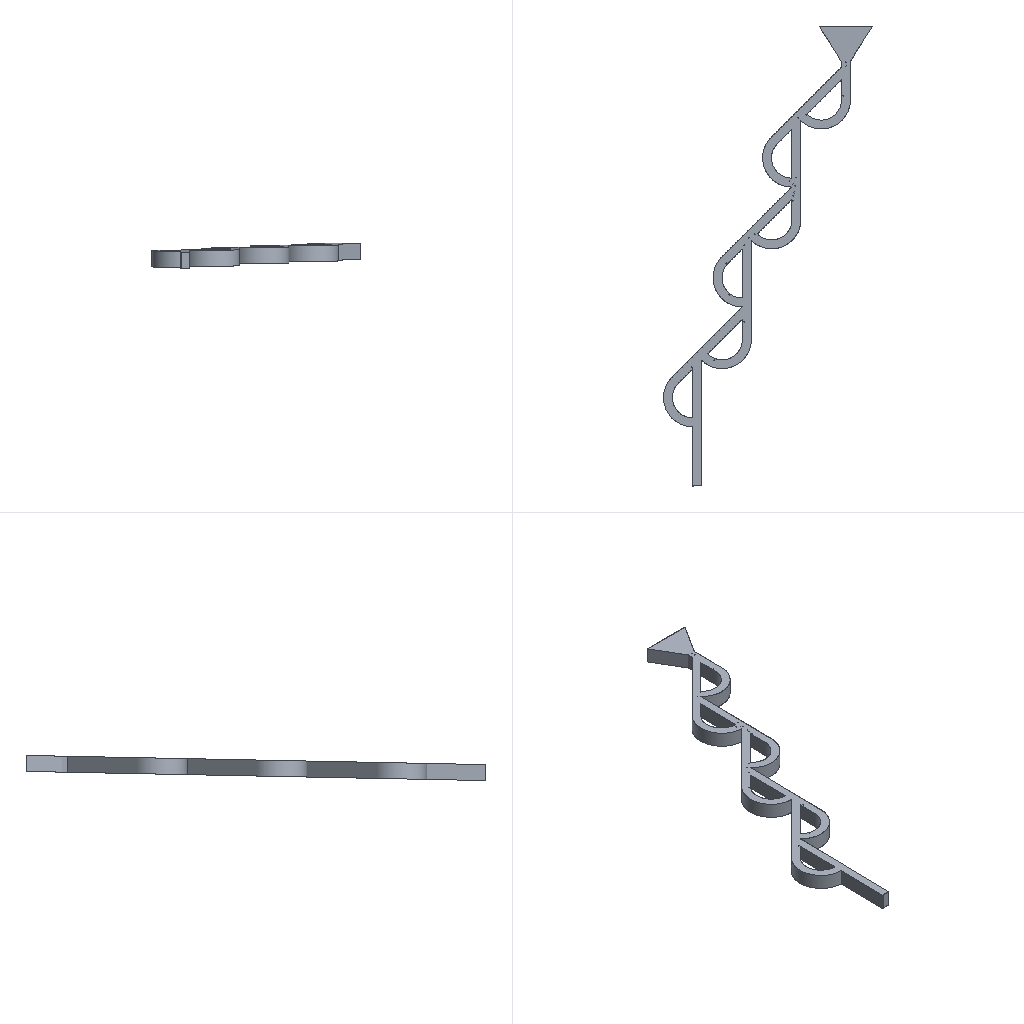Simulation study | ansys fluent
Set-up summary:
category,name,step,type,value,unit,region
solver,ansys_fluent,,Fluent 26.1.0
units,SI m-kg-s (Fluent internal),,stated,boundary values in the units shown in brackets; results in listed units
analysis,deck.cas,,cfd steady,"dimension=3D; solver=3d, dp, pbns, vof, rngke (3d, double precision, pressure-based, VOF, RNG k-epsilon); source_case=.cas"
model,Space,deck.cas,,3D
model,Time,deck.cas,,Steady
model,Viscous,deck.cas,,RNG k-epsilon turbulence model
model,Wall Treatment,deck.cas,,Standard Wall Functions
model,Heat Transfer,deck.cas,,Disabled
model,Multiphase,deck.cas,,Volume of Fluid
mesh,nodes,,,267140
mesh,elements,,,233262
mesh,faces,,,732653
cell_zone,part_1 (mixture),deck.cas,fluid,material=water-liquid,,zone 3
cell_zone,part_1 (air),deck.cas,fluid,material=air,,zone 3
cell_zone,part_1 (water),deck.cas,fluid,material=water-liquid,,zone 3
material,water-liquid (fluid),,Density,998.2,kg/m^3
material,water-liquid (fluid),,Viscosity,0.001003,kg/(m s)
material,air (fluid),,Density,1.225,kg/m^3
material,air (fluid),,Viscosity,1.7894e-05,kg/(m s)
material,aluminum (solid),,Density,2719,kg/m^3
bc,out1 (mixture),deck.cas,pressure-outlet,Backflow Direction Specification Method=Normal to Boundary,,zone 7
bc,out1 (air),deck.cas,pressure-outlet,,,zone 7
bc,out1 (water),deck.cas,pressure-outlet,,,zone 7
bc,int (mixture),deck.cas,velocity-inlet,Velocity Magnitude [m/s]=0.05,,zone 6
bc,int (air),deck.cas,velocity-inlet,,,zone 6
bc,int (water),deck.cas,velocity-inlet,Volume Fraction=1,,zone 6
bc,wall-part_1 (mixture),deck.cas,wall,Wall Motion=Stationary Wall; Shear Boundary Condition=No Slip,,zone 1
bc,wall-part_1 (air),deck.cas,wall,,,zone 1
bc,wall-part_1 (water),deck.cas,wall,,,zone 1
bc,wall (mixture),deck.cas,wall,Wall Motion=Stationary Wall; Shear Boundary Condition=No Slip,,zone 8
bc,wall (air),deck.cas,wall,,,zone 8
bc,wall (water),deck.cas,wall,,,zone 8
bc,out (mixture),deck.cas,pressure-outlet,Backflow Direction Specification Method=Normal to Boundary,,zone 9
bc,out (air),deck.cas,pressure-outlet,,,zone 9
bc,out (water),deck.cas,pressure-outlet,,,zone 9
Results summary:
result,mass flow rate int,deck.cas,,539.028,kg/s
result,mass flow rate out,deck.cas,,-224.243,kg/s
result,mass flow rate out1,deck.cas,,-222.697,kg/s
result,mass flow rate wall,deck.cas,,-0,kg/s
result,mass flow rate wall-part_1,deck.cas,,-0,kg/s
result,mass flow rate Net,deck.cas,,92.088,kg/s
result,wall force total wall,deck.cas,,"(225.507, -13968.3, -770411)",N
result,wall force pressure wall,deck.cas,,"(287.845, -13814.9, -770423)",N
result,wall force viscous wall,deck.cas,,"(-62.338, -153.401, 12.77)",N
result,wall force total wall-part_1,deck.cas,,"(-228.374, 7077.63, 4.063)",N
result,wall force pressure wall-part_1,deck.cas,,"(-220.798, 7097.53, 7.1624e-06)",N
result,wall force viscous wall-part_1,deck.cas,,"(-7.576, -19.898, 4.063)",N
result,wall force total Net,deck.cas,,"(-2.867, -6890.63, -770407)",N
result,wall force pressure Net,deck.cas,,"(67.047, -6717.33, -770423)",N
result,wall force viscous Net,deck.cas,,"(-69.914, -173.299, 16.833)",N